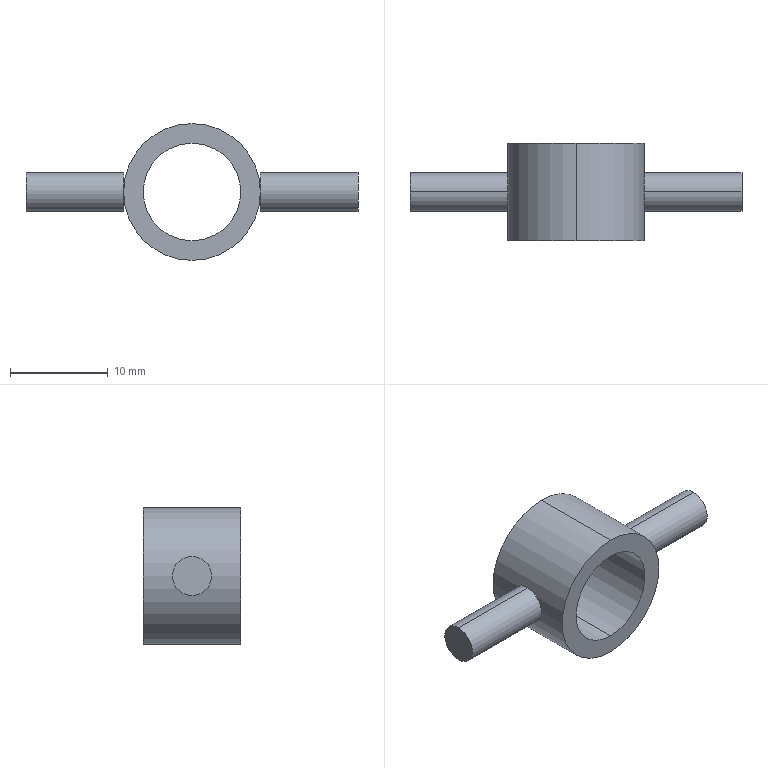Part | SolidWorks | features Extrusion 1, ICE 1, MirrorSolid 1 | 3 solids | 14 faces | box 34 x 10 x 14 mm | volume 1005 mm3 | cylinder 8 | plane 6 | commonest cylinder face diameters 4 x4 10 x2 14 x2
STEP:
#1=CARTESIAN_POINT('',(0.,10.,-5.));
#2=VERTEX_POINT('',#1);
#3=CARTESIAN_POINT('',(0.,10.,5.));
#4=VERTEX_POINT('',#3);
#5=CARTESIAN_POINT('',(0.,10.,0.));
#6=DIRECTION('',(0.,1.,0.));
#7=DIRECTION('',(0.,0.,1.));
#8=AXIS2_PLACEMENT_3D('',#5,#6,#7);
#9=CIRCLE('',#8,5.);
#10=EDGE_CURVE('',#2,#4,#9,.T.);
#11=ORIENTED_EDGE('',*,*,#10,.T.);
#12=CARTESIAN_POINT('',(0.,0.,5.));
#13=VERTEX_POINT('',#12);
#14=CARTESIAN_POINT('',(0.,10.,5.));
#15=DIRECTION('',(0.,-1.,0.));
#16=VECTOR('',#15,1000.);
#17=LINE('',#14,#16);
#18=EDGE_CURVE('',#4,#13,#17,.T.);
#19=ORIENTED_EDGE('',*,*,#18,.T.);
#20=CARTESIAN_POINT('',(0.,0.,-5.));
#21=VERTEX_POINT('',#20);
#22=CARTESIAN_POINT('',(0.,0.,0.));
#23=DIRECTION('',(0.,1.,0.));
#24=DIRECTION('',(0.,0.,1.));
#25=AXIS2_PLACEMENT_3D('',#22,#23,#24);
#26=CIRCLE('',#25,5.);
#27=EDGE_CURVE('',#21,#13,#26,.T.);
#28=ORIENTED_EDGE('',*,*,#27,.F.);
#29=CARTESIAN_POINT('',(0.,10.,-5.));
#30=DIRECTION('',(0.,-1.,0.));
#31=VECTOR('',#30,1000.);
#32=LINE('',#29,#31);
#33=EDGE_CURVE('',#2,#21,#32,.T.);
#34=ORIENTED_EDGE('',*,*,#33,.F.);
#35=EDGE_LOOP('',(#11,#19,#28,#34));
#36=FACE_OUTER_BOUND('',#35,.T.);
#37=CARTESIAN_POINT('',(0.,10.,0.));
#38=DIRECTION('',(0.,-1.,0.));
#39=DIRECTION('',(0.,0.,-1.));
#40=AXIS2_PLACEMENT_3D('',#37,#38,#39);
#41=CYLINDRICAL_SURFACE('',#40,5.);
#42=ADVANCED_FACE('',(#36),#41,.F.);
#43=CARTESIAN_POINT('',(0.,10.,7.));
#44=VERTEX_POINT('',#43);
#45=CARTESIAN_POINT('',(0.,10.,-7.));
#46=VERTEX_POINT('',#45);
#47=CARTESIAN_POINT('',(0.,10.,0.));
#48=DIRECTION('',(0.,1.,0.));
#49=DIRECTION('',(0.,0.,1.));
#50=AXIS2_PLACEMENT_3D('',#47,#48,#49);
#51=CIRCLE('',#50,7.);
#52=EDGE_CURVE('',#44,#46,#51,.T.);
#53=ORIENTED_EDGE('',*,*,#52,.F.);
#54=CARTESIAN_POINT('',(0.,0.,7.));
#55=VERTEX_POINT('',#54);
#56=CARTESIAN_POINT('',(0.,10.,7.));
#57=DIRECTION('',(0.,-1.,0.));
#58=VECTOR('',#57,1000.);
#59=LINE('',#56,#58);
#60=EDGE_CURVE('',#44,#55,#59,.T.);
#61=ORIENTED_EDGE('',*,*,#60,.T.);
#62=CARTESIAN_POINT('',(0.,0.,-7.));
#63=VERTEX_POINT('',#62);
#64=CARTESIAN_POINT('',(0.,0.,0.));
#65=DIRECTION('',(0.,1.,0.));
#66=DIRECTION('',(0.,0.,1.));
#67=AXIS2_PLACEMENT_3D('',#64,#65,#66);
#68=CIRCLE('',#67,7.);
#69=EDGE_CURVE('',#55,#63,#68,.T.);
#70=ORIENTED_EDGE('',*,*,#69,.T.);
#71=CARTESIAN_POINT('',(0.,10.,-7.));
#72=DIRECTION('',(0.,-1.,0.));
#73=VECTOR('',#72,1000.);
#74=LINE('',#71,#73);
#75=EDGE_CURVE('',#46,#63,#74,.T.);
#76=ORIENTED_EDGE('',*,*,#75,.F.);
#77=EDGE_LOOP('',(#53,#61,#70,#76));
#78=FACE_OUTER_BOUND('',#77,.T.);
#79=CARTESIAN_POINT('',(0.,10.,0.));
#80=DIRECTION('',(0.,-1.,0.));
#81=DIRECTION('',(0.,0.,-1.));
#82=AXIS2_PLACEMENT_3D('',#79,#80,#81);
#83=CYLINDRICAL_SURFACE('',#82,7.);
#84=ADVANCED_FACE('',(#78),#83,.T.);
#85=CARTESIAN_POINT('',(0.,10.,0.));
#86=DIRECTION('',(0.,1.,0.));
#87=DIRECTION('',(0.,0.,1.));
#88=AXIS2_PLACEMENT_3D('',#85,#86,#87);
#89=CIRCLE('',#88,7.);
#90=EDGE_CURVE('',#46,#44,#89,.T.);
#91=ORIENTED_EDGE('',*,*,#90,.T.);
#92=ORIENTED_EDGE('',*,*,#52,.T.);
#93=EDGE_LOOP('',(#91,#92));
#94=FACE_OUTER_BOUND('',#93,.T.);
#95=ORIENTED_EDGE('',*,*,#10,.F.);
#96=CARTESIAN_POINT('',(0.,10.,0.));
#97=DIRECTION('',(0.,1.,0.));
#98=DIRECTION('',(0.,0.,1.));
#99=AXIS2_PLACEMENT_3D('',#96,#97,#98);
#100=CIRCLE('',#99,5.);
#101=EDGE_CURVE('',#4,#2,#100,.T.);
#102=ORIENTED_EDGE('',*,*,#101,.F.);
#103=EDGE_LOOP('',(#95,#102));
#104=FACE_BOUND('',#103,.T.);
#105=CARTESIAN_POINT('',(0.,10.,0.));
#106=DIRECTION('',(0.,1.,0.));
#107=DIRECTION('',(0.,0.,1.));
#108=AXIS2_PLACEMENT_3D('',#105,#106,#107);
#109=PLANE('',#108);
#110=ADVANCED_FACE('',(#94,#104),#109,.T.);
#111=CARTESIAN_POINT('',(0.,0.,0.));
#112=DIRECTION('',(0.,1.,0.));
#113=DIRECTION('',(0.,0.,1.));
#114=AXIS2_PLACEMENT_3D('',#111,#112,#113);
#115=CIRCLE('',#114,7.);
#116=EDGE_CURVE('',#63,#55,#115,.T.);
#117=ORIENTED_EDGE('',*,*,#116,.F.);
#118=ORIENTED_EDGE('',*,*,#69,.F.);
#119=EDGE_LOOP('',(#117,#118));
#120=FACE_OUTER_BOUND('',#119,.T.);
#121=ORIENTED_EDGE('',*,*,#27,.T.);
#122=CARTESIAN_POINT('',(0.,0.,0.));
#123=DIRECTION('',(0.,1.,0.));
#124=DIRECTION('',(0.,0.,1.));
#125=AXIS2_PLACEMENT_3D('',#122,#123,#124);
#126=CIRCLE('',#125,5.);
#127=EDGE_CURVE('',#13,#21,#126,.T.);
#128=ORIENTED_EDGE('',*,*,#127,.T.);
#129=EDGE_LOOP('',(#121,#128));
#130=FACE_BOUND('',#129,.T.);
#131=CARTESIAN_POINT('',(0.,0.,0.));
#132=DIRECTION('',(0.,1.,0.));
#133=DIRECTION('',(0.,0.,1.));
#134=AXIS2_PLACEMENT_3D('',#131,#132,#133);
#135=PLANE('',#134);
#136=ADVANCED_FACE('',(#120,#130),#135,.F.);
#137=ORIENTED_EDGE('',*,*,#60,.F.);
#138=ORIENTED_EDGE('',*,*,#90,.F.);
#139=ORIENTED_EDGE('',*,*,#75,.T.);
#140=ORIENTED_EDGE('',*,*,#116,.T.);
#141=EDGE_LOOP('',(#137,#138,#139,#140));
#142=FACE_OUTER_BOUND('',#141,.T.);
#143=CARTESIAN_POINT('',(0.,10.,0.));
#144=DIRECTION('',(0.,-1.,0.));
#145=DIRECTION('',(0.,0.,-1.));
#146=AXIS2_PLACEMENT_3D('',#143,#144,#145);
#147=CYLINDRICAL_SURFACE('',#146,7.);
#148=ADVANCED_FACE('',(#142),#147,.T.);
#149=ORIENTED_EDGE('',*,*,#18,.F.);
#150=ORIENTED_EDGE('',*,*,#101,.T.);
#151=ORIENTED_EDGE('',*,*,#33,.T.);
#152=ORIENTED_EDGE('',*,*,#127,.F.);
#153=EDGE_LOOP('',(#149,#150,#151,#152));
#154=FACE_OUTER_BOUND('',#153,.T.);
#155=CARTESIAN_POINT('',(0.,10.,0.));
#156=DIRECTION('',(0.,-1.,0.));
#157=DIRECTION('',(0.,0.,-1.));
#158=AXIS2_PLACEMENT_3D('',#155,#156,#157);
#159=CYLINDRICAL_SURFACE('',#158,5.);
#160=ADVANCED_FACE('',(#154),#159,.F.);
#161=CLOSED_SHELL('',(#42,#84,#110,#136,#148,#160));
#162=MANIFOLD_SOLID_BREP('',#161);
#163=CARTESIAN_POINT('',(-17.,5.,2.));
#164=VERTEX_POINT('',#163);
#165=CARTESIAN_POINT('',(-17.,5.,-2.));
#166=VERTEX_POINT('',#165);
#167=CARTESIAN_POINT('',(-17.,5.,0.));
#168=DIRECTION('',(-1.,0.,0.));
#169=DIRECTION('',(0.,0.,1.));
#170=AXIS2_PLACEMENT_3D('',#167,#168,#169);
#171=CIRCLE('',#170,2.);
#172=EDGE_CURVE('',#164,#166,#171,.T.);
#173=ORIENTED_EDGE('',*,*,#172,.F.);
#174=CARTESIAN_POINT('',(-7.,5.,2.));
#175=VERTEX_POINT('',#174);
#176=CARTESIAN_POINT('',(-17.,5.,2.));
#177=DIRECTION('',(1.,0.,0.));
#178=VECTOR('',#177,1000.);
#179=LINE('',#176,#178);
#180=EDGE_CURVE('',#164,#175,#179,.T.);
#181=ORIENTED_EDGE('',*,*,#180,.T.);
#182=CARTESIAN_POINT('',(-7.,5.,-2.));
#183=VERTEX_POINT('',#182);
#184=CARTESIAN_POINT('',(-7.,5.,0.));
#185=DIRECTION('',(-1.,0.,0.));
#186=DIRECTION('',(0.,0.,1.));
#187=AXIS2_PLACEMENT_3D('',#184,#185,#186);
#188=CIRCLE('',#187,2.);
#189=EDGE_CURVE('',#175,#183,#188,.T.);
#190=ORIENTED_EDGE('',*,*,#189,.T.);
#191=CARTESIAN_POINT('',(-17.,5.,-2.));
#192=DIRECTION('',(1.,0.,0.));
#193=VECTOR('',#192,1000.);
#194=LINE('',#191,#193);
#195=EDGE_CURVE('',#166,#183,#194,.T.);
#196=ORIENTED_EDGE('',*,*,#195,.F.);
#197=EDGE_LOOP('',(#173,#181,#190,#196));
#198=FACE_OUTER_BOUND('',#197,.T.);
#199=CARTESIAN_POINT('',(-17.,5.,0.));
#200=DIRECTION('',(1.,0.,0.));
#201=DIRECTION('',(0.,0.,-1.));
#202=AXIS2_PLACEMENT_3D('',#199,#200,#201);
#203=CYLINDRICAL_SURFACE('',#202,2.);
#204=ADVANCED_FACE('',(#198),#203,.T.);
#205=ORIENTED_EDGE('',*,*,#180,.F.);
#206=CARTESIAN_POINT('',(-17.,5.,0.));
#207=DIRECTION('',(-1.,0.,0.));
#208=DIRECTION('',(0.,0.,1.));
#209=AXIS2_PLACEMENT_3D('',#206,#207,#208);
#210=CIRCLE('',#209,2.);
#211=EDGE_CURVE('',#166,#164,#210,.T.);
#212=ORIENTED_EDGE('',*,*,#211,.F.);
#213=ORIENTED_EDGE('',*,*,#195,.T.);
#214=CARTESIAN_POINT('',(-7.,5.,0.));
#215=DIRECTION('',(-1.,0.,0.));
#216=DIRECTION('',(0.,0.,1.));
#217=AXIS2_PLACEMENT_3D('',#214,#215,#216);
#218=CIRCLE('',#217,2.);
#219=EDGE_CURVE('',#183,#175,#218,.T.);
#220=ORIENTED_EDGE('',*,*,#219,.T.);
#221=EDGE_LOOP('',(#205,#212,#213,#220));
#222=FACE_OUTER_BOUND('',#221,.T.);
#223=CARTESIAN_POINT('',(-17.,5.,0.));
#224=DIRECTION('',(1.,0.,0.));
#225=DIRECTION('',(0.,0.,-1.));
#226=AXIS2_PLACEMENT_3D('',#223,#224,#225);
#227=CYLINDRICAL_SURFACE('',#226,2.);
#228=ADVANCED_FACE('',(#222),#227,.T.);
#229=ORIENTED_EDGE('',*,*,#211,.T.);
#230=ORIENTED_EDGE('',*,*,#172,.T.);
#231=EDGE_LOOP('',(#229,#230));
#232=FACE_OUTER_BOUND('',#231,.T.);
#233=CARTESIAN_POINT('',(-17.,5.,0.));
#234=DIRECTION('',(-1.,0.,0.));
#235=DIRECTION('',(0.,0.,1.));
#236=AXIS2_PLACEMENT_3D('',#233,#234,#235);
#237=PLANE('',#236);
#238=ADVANCED_FACE('',(#232),#237,.T.);
#239=ORIENTED_EDGE('',*,*,#219,.F.);
#240=ORIENTED_EDGE('',*,*,#189,.F.);
#241=EDGE_LOOP('',(#239,#240));
#242=FACE_OUTER_BOUND('',#241,.T.);
#243=CARTESIAN_POINT('',(-7.,5.,0.));
#244=DIRECTION('',(-1.,0.,0.));
#245=DIRECTION('',(0.,0.,1.));
#246=AXIS2_PLACEMENT_3D('',#243,#244,#245);
#247=PLANE('',#246);
#248=ADVANCED_FACE('',(#242),#247,.F.);
#249=CLOSED_SHELL('',(#204,#228,#238,#248));
#250=MANIFOLD_SOLID_BREP('',#249);
#251=CARTESIAN_POINT('',(17.,5.,-2.));
#252=VERTEX_POINT('',#251);
#253=CARTESIAN_POINT('',(17.,5.,2.));
#254=VERTEX_POINT('',#253);
#255=CARTESIAN_POINT('',(17.,5.,0.));
#256=DIRECTION('',(-1.,0.,0.));
#257=DIRECTION('',(0.,0.,1.));
#258=AXIS2_PLACEMENT_3D('',#255,#256,#257);
#259=CIRCLE('',#258,2.);
#260=EDGE_CURVE('',#252,#254,#259,.T.);
#261=ORIENTED_EDGE('',*,*,#260,.T.);
#262=CARTESIAN_POINT('',(7.,5.,2.));
#263=VERTEX_POINT('',#262);
#264=CARTESIAN_POINT('',(17.,5.,2.));
#265=DIRECTION('',(-1.,0.,0.));
#266=VECTOR('',#265,1000.);
#267=LINE('',#264,#266);
#268=EDGE_CURVE('',#254,#263,#267,.T.);
#269=ORIENTED_EDGE('',*,*,#268,.T.);
#270=CARTESIAN_POINT('',(7.,5.,-2.));
#271=VERTEX_POINT('',#270);
#272=CARTESIAN_POINT('',(7.,5.,0.));
#273=DIRECTION('',(-1.,0.,0.));
#274=DIRECTION('',(0.,0.,1.));
#275=AXIS2_PLACEMENT_3D('',#272,#273,#274);
#276=CIRCLE('',#275,2.);
#277=EDGE_CURVE('',#271,#263,#276,.T.);
#278=ORIENTED_EDGE('',*,*,#277,.F.);
#279=CARTESIAN_POINT('',(17.,5.,-2.));
#280=DIRECTION('',(-1.,0.,0.));
#281=VECTOR('',#280,1000.);
#282=LINE('',#279,#281);
#283=EDGE_CURVE('',#252,#271,#282,.T.);
#284=ORIENTED_EDGE('',*,*,#283,.F.);
#285=EDGE_LOOP('',(#261,#269,#278,#284));
#286=FACE_OUTER_BOUND('',#285,.T.);
#287=CARTESIAN_POINT('',(17.,5.,0.));
#288=DIRECTION('',(-1.,0.,0.));
#289=DIRECTION('',(0.,0.,-1.));
#290=AXIS2_PLACEMENT_3D('',#287,#288,#289);
#291=CYLINDRICAL_SURFACE('',#290,2.);
#292=ADVANCED_FACE('',(#286),#291,.T.);
#293=ORIENTED_EDGE('',*,*,#268,.F.);
#294=CARTESIAN_POINT('',(17.,5.,0.));
#295=DIRECTION('',(-1.,0.,0.));
#296=DIRECTION('',(0.,0.,1.));
#297=AXIS2_PLACEMENT_3D('',#294,#295,#296);
#298=CIRCLE('',#297,2.);
#299=EDGE_CURVE('',#254,#252,#298,.T.);
#300=ORIENTED_EDGE('',*,*,#299,.T.);
#301=ORIENTED_EDGE('',*,*,#283,.T.);
#302=CARTESIAN_POINT('',(7.,5.,0.));
#303=DIRECTION('',(-1.,0.,0.));
#304=DIRECTION('',(0.,0.,1.));
#305=AXIS2_PLACEMENT_3D('',#302,#303,#304);
#306=CIRCLE('',#305,2.);
#307=EDGE_CURVE('',#263,#271,#306,.T.);
#308=ORIENTED_EDGE('',*,*,#307,.F.);
#309=EDGE_LOOP('',(#293,#300,#301,#308));
#310=FACE_OUTER_BOUND('',#309,.T.);
#311=CARTESIAN_POINT('',(17.,5.,0.));
#312=DIRECTION('',(-1.,0.,0.));
#313=DIRECTION('',(0.,0.,-1.));
#314=AXIS2_PLACEMENT_3D('',#311,#312,#313);
#315=CYLINDRICAL_SURFACE('',#314,2.);
#316=ADVANCED_FACE('',(#310),#315,.T.);
#317=ORIENTED_EDGE('',*,*,#260,.F.);
#318=ORIENTED_EDGE('',*,*,#299,.F.);
#319=EDGE_LOOP('',(#317,#318));
#320=FACE_OUTER_BOUND('',#319,.T.);
#321=CARTESIAN_POINT('',(17.,5.,0.));
#322=DIRECTION('',(1.,0.,0.));
#323=DIRECTION('',(0.,0.,1.));
#324=AXIS2_PLACEMENT_3D('',#321,#322,#323);
#325=PLANE('',#324);
#326=ADVANCED_FACE('',(#320),#325,.T.);
#327=ORIENTED_EDGE('',*,*,#277,.T.);
#328=ORIENTED_EDGE('',*,*,#307,.T.);
#329=EDGE_LOOP('',(#327,#328));
#330=FACE_OUTER_BOUND('',#329,.T.);
#331=CARTESIAN_POINT('',(7.,5.,0.));
#332=DIRECTION('',(1.,0.,0.));
#333=DIRECTION('',(0.,0.,1.));
#334=AXIS2_PLACEMENT_3D('',#331,#332,#333);
#335=PLANE('',#334);
#336=ADVANCED_FACE('',(#330),#335,.F.);
#337=CLOSED_SHELL('',(#292,#316,#326,#336));
#338=MANIFOLD_SOLID_BREP('',#337);
#339=CARTESIAN_POINT('',(0.,0.,0.));
#340=DIRECTION('',(0.,0.,1.));
#341=DIRECTION('',(1.,0.,0.));
#342=AXIS2_PLACEMENT_3D('',#339,#340,#341);
#343=(LENGTH_UNIT()NAMED_UNIT(*)SI_UNIT(.MILLI.,.METRE.));
#344=UNCERTAINTY_MEASURE_WITH_UNIT(LENGTH_MEASURE(0.00001),#343,'','');
#345=(NAMED_UNIT(*)PLANE_ANGLE_UNIT()SI_UNIT($,.RADIAN.));
#346=(NAMED_UNIT(*)SI_UNIT($,.STERADIAN.)SOLID_ANGLE_UNIT());
#347=(GEOMETRIC_REPRESENTATION_CONTEXT(3)GLOBAL_UNCERTAINTY_ASSIGNED_CONTEXT((#344))GLOBAL_UNIT_ASSIGNED_CONTEXT((#343,#345,#346))REPRESENTATION_CONTEXT('',''));
#348=ADVANCED_BREP_SHAPE_REPRESENTATION('',(#162,#250,#338,#342),#347);